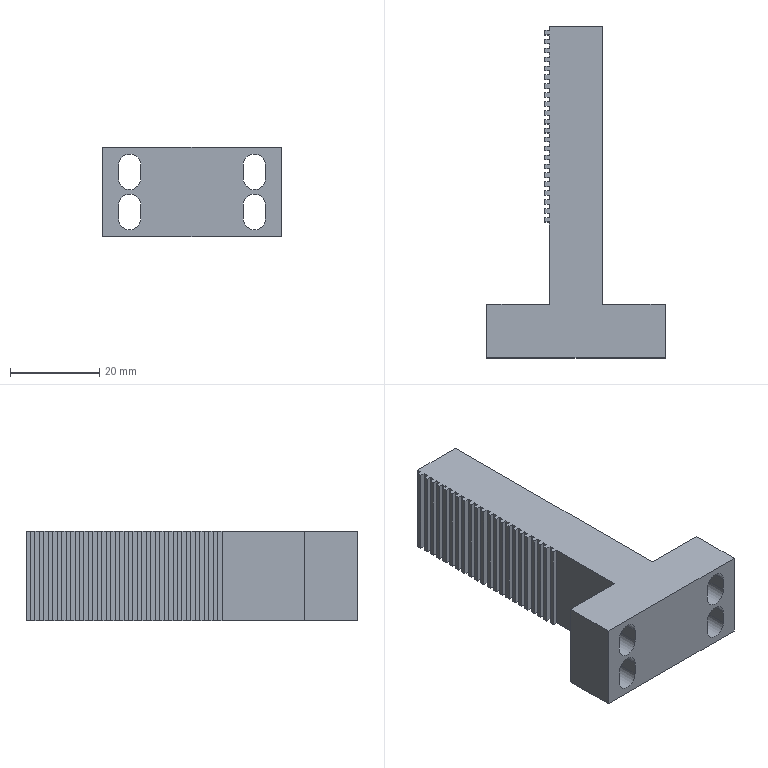Part | SolidWorks | features ICE 2, Extrusion 1, LPattern 1 | 1 solid | 118 faces | box 40 x 74.5 x 20 mm | volume 23378 mm3 | plane 106 | cylinder 12 | commonest cylinder face diameters 5 x12